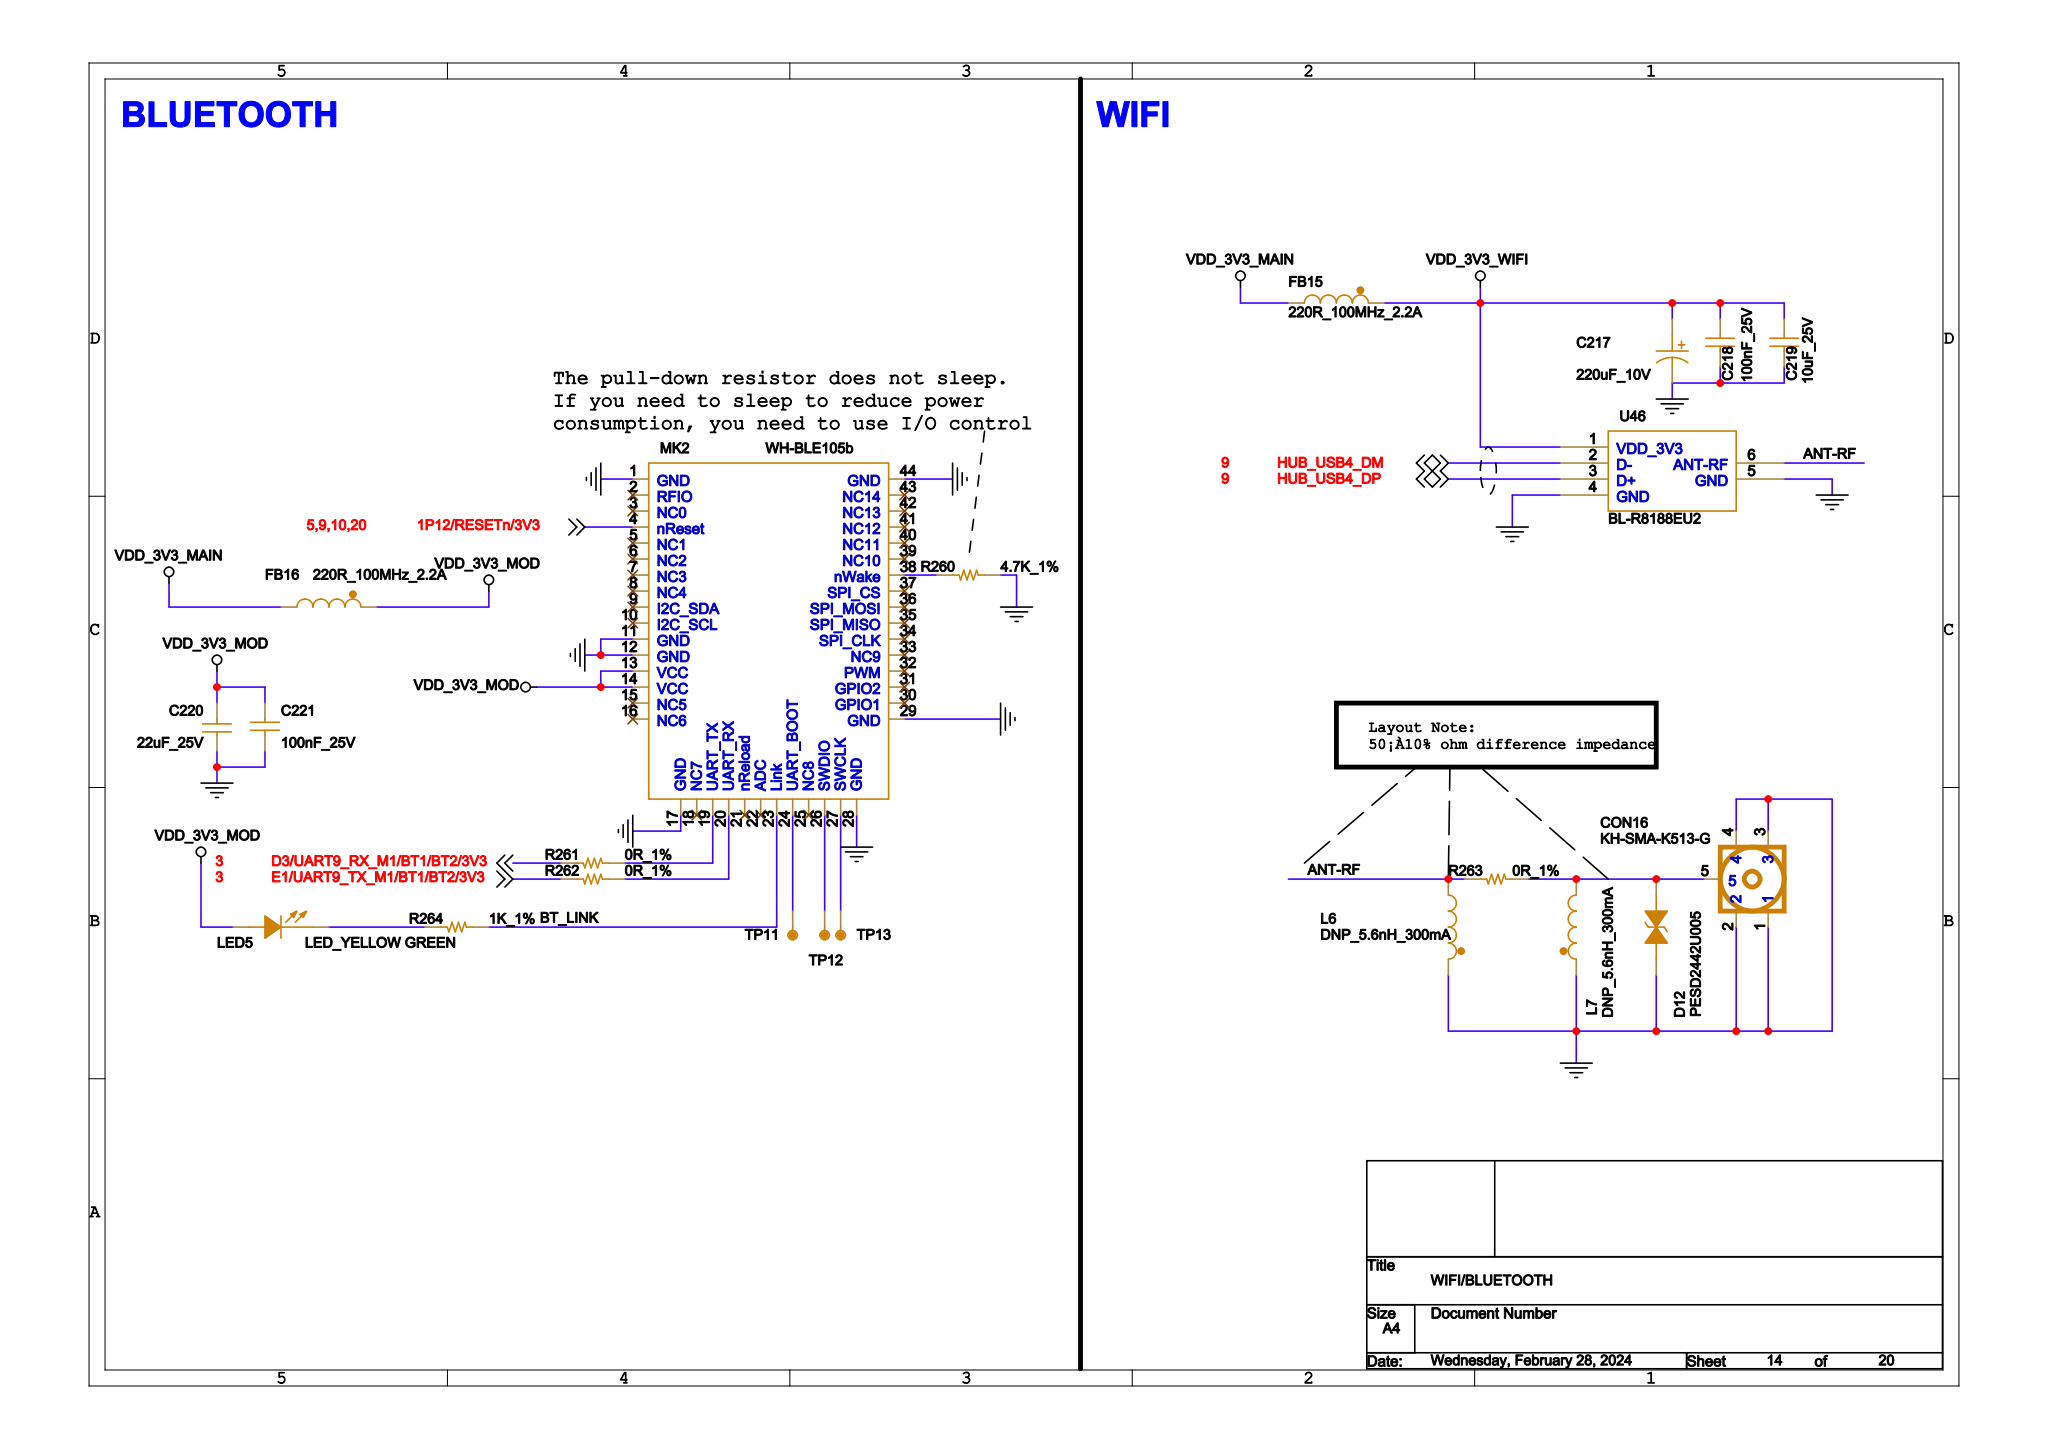Circuit board | Cadence Allegro | 1024 parts | 682 nets | one sheet of the schematic
Parts on this sheet (reference | value | footprint):
C217 | 220uF_10V | CAP_CASE_D
C219 | 10uF_25V | C0603
C220 | 22uF_25V | C0805
C221 | 100nF_25V | C0402
CON16 | KH-SMA-K513-G | CON_SMA_5P_V_DIP
D12 | PESD2442U005 | ESD_0402
FB15 | 220R_100MHz_2A | L0603
FB16 | 220R_100MHz_2A | L0603
L6 | DNP_5.6nH_300mA | L0402
L7 | DNP_5.6nH_300mA | L0402
LED5 | LED_GREEN | D0603
MK2 | WH-BLE105 | SMD_44P_1822X2680_WH-BLE105
R260 | 4.7K_1% | R0402
R261 | 0R_1% | R0402
R262 | 0R_1% | R0402
R263 | 0R_1% | R0402
R264 | 1K_1% | R0402
TP11 | SMT TP | TP30
TP12 | SMT TP | TP30
TP13 | SMT TP | TP30
U46 | BL-R8188EU2 | SMD_6P_13X12D3_BL-RTL8188EUS
Nets of these parts (net: part-pin ...):
GND: C217-2 C219-2 C220-1 C221-2 CON16-1 CON16-2 CON16-3 CON16-4 D12-2 L6-1 L7-1 MK2-1 MK2-11 MK2-12 MK2-17 MK2-28 MK2-29 MK2-44 R260-2 U46-4 U46-5
VDD_3V3_MAIN: FB15-2 FB16-2
1P12/RESETN/3V3: MK2-4
E1/UART9_TX_M1/BT1/BT2/3V3: R262-1
D3/UART9_RX_M1/BT1/BT2/3V3: R261-1
N21614292: CON16-5 D12-1 L7-2 R263-2
BT_LINK: MK2-23 R264-1
N21613689: LED5-2 R264-2
N21613876: MK2-38 R260-1
VDD_3V3_WIFI: C217-1 C219-1 FB15-1 U46-1
ANT-RF: L6-2 R263-1 U46-6
N21613714: MK2-19 R261-2
N21613683: MK2-20 R262-2
VDD_3V3_MOD: C220-2 C221-1 FB16-1 LED5-1 MK2-13 MK2-14
N21613874: MK2-27 TP13-1
N21613872: MK2-26 TP12-1
N21613880: MK2-24 TP11-1
HUB_USB4_DP: U46-3
HUB_USB4_DM: U46-2